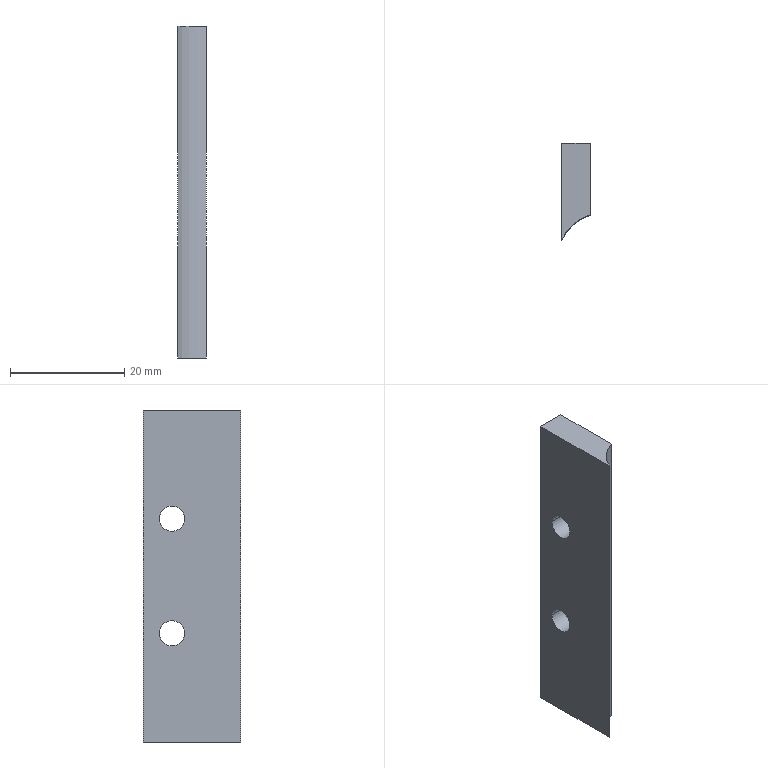Part | SolidWorks | features Extrusion 1, ICE 1 | 1 solid | 10 faces | box 5 x 17 x 58 mm | volume 3929 mm3 | cylinder 5 | plane 5 | commonest cylinder face diameters 4.4 x4 15.6 x1
STEP:
#1=CARTESIAN_POINT('',(-3.012,-2.658,19.));
#2=VERTEX_POINT('',#1);
#3=CARTESIAN_POINT('',(-3.012,1.742,19.));
#4=VERTEX_POINT('',#3);
#5=CARTESIAN_POINT('',(-3.012,-0.4585,19.));
#6=DIRECTION('',(1.,0.,0.));
#7=DIRECTION('',(0.,1.,0.));
#8=AXIS2_PLACEMENT_3D('',#5,#6,#7);
#9=CIRCLE('',#8,2.2);
#10=EDGE_CURVE('',#2,#4,#9,.T.);
#11=ORIENTED_EDGE('',*,*,#10,.F.);
#12=CARTESIAN_POINT('',(1.988,-2.658,19.));
#13=VERTEX_POINT('',#12);
#14=CARTESIAN_POINT('',(-8.012,-2.658,19.));
#15=DIRECTION('',(1.,0.,0.));
#16=VECTOR('',#15,1000.);
#17=LINE('',#14,#16);
#18=EDGE_CURVE('',#2,#13,#17,.T.);
#19=ORIENTED_EDGE('',*,*,#18,.T.);
#20=CARTESIAN_POINT('',(1.988,1.742,19.));
#21=VERTEX_POINT('',#20);
#22=CARTESIAN_POINT('',(1.988,-0.4585,19.));
#23=DIRECTION('',(1.,0.,0.));
#24=DIRECTION('',(0.,1.,0.));
#25=AXIS2_PLACEMENT_3D('',#22,#23,#24);
#26=CIRCLE('',#25,2.2);
#27=EDGE_CURVE('',#13,#21,#26,.T.);
#28=ORIENTED_EDGE('',*,*,#27,.T.);
#29=CARTESIAN_POINT('',(-8.012,1.742,19.));
#30=DIRECTION('',(1.,0.,0.));
#31=VECTOR('',#30,1000.);
#32=LINE('',#29,#31);
#33=EDGE_CURVE('',#4,#21,#32,.T.);
#34=ORIENTED_EDGE('',*,*,#33,.F.);
#35=EDGE_LOOP('',(#11,#19,#28,#34));
#36=FACE_OUTER_BOUND('',#35,.T.);
#37=CARTESIAN_POINT('',(-8.012,-0.4585,19.));
#38=DIRECTION('',(1.,0.,0.));
#39=DIRECTION('',(0.,1.,0.));
#40=AXIS2_PLACEMENT_3D('',#37,#38,#39);
#41=CYLINDRICAL_SURFACE('',#40,2.2);
#42=ADVANCED_FACE('',(#36),#41,.F.);
#43=CARTESIAN_POINT('',(-3.012,-2.658,39.));
#44=VERTEX_POINT('',#43);
#45=CARTESIAN_POINT('',(-3.012,1.742,39.));
#46=VERTEX_POINT('',#45);
#47=CARTESIAN_POINT('',(-3.012,-0.4585,39.));
#48=DIRECTION('',(1.,0.,0.));
#49=DIRECTION('',(0.,1.,0.));
#50=AXIS2_PLACEMENT_3D('',#47,#48,#49);
#51=CIRCLE('',#50,2.2);
#52=EDGE_CURVE('',#44,#46,#51,.T.);
#53=ORIENTED_EDGE('',*,*,#52,.F.);
#54=CARTESIAN_POINT('',(1.988,-2.658,39.));
#55=VERTEX_POINT('',#54);
#56=CARTESIAN_POINT('',(-8.012,-2.658,39.));
#57=DIRECTION('',(1.,0.,0.));
#58=VECTOR('',#57,1000.);
#59=LINE('',#56,#58);
#60=EDGE_CURVE('',#44,#55,#59,.T.);
#61=ORIENTED_EDGE('',*,*,#60,.T.);
#62=CARTESIAN_POINT('',(1.988,1.742,39.));
#63=VERTEX_POINT('',#62);
#64=CARTESIAN_POINT('',(1.988,-0.4585,39.));
#65=DIRECTION('',(1.,0.,0.));
#66=DIRECTION('',(0.,1.,0.));
#67=AXIS2_PLACEMENT_3D('',#64,#65,#66);
#68=CIRCLE('',#67,2.2);
#69=EDGE_CURVE('',#55,#63,#68,.T.);
#70=ORIENTED_EDGE('',*,*,#69,.T.);
#71=CARTESIAN_POINT('',(-8.012,1.742,39.));
#72=DIRECTION('',(1.,0.,0.));
#73=VECTOR('',#72,1000.);
#74=LINE('',#71,#73);
#75=EDGE_CURVE('',#46,#63,#74,.T.);
#76=ORIENTED_EDGE('',*,*,#75,.F.);
#77=EDGE_LOOP('',(#53,#61,#70,#76));
#78=FACE_OUTER_BOUND('',#77,.T.);
#79=CARTESIAN_POINT('',(-8.012,-0.4585,39.));
#80=DIRECTION('',(1.,0.,0.));
#81=DIRECTION('',(0.,1.,0.));
#82=AXIS2_PLACEMENT_3D('',#79,#80,#81);
#83=CYLINDRICAL_SURFACE('',#82,2.2);
#84=ADVANCED_FACE('',(#78),#83,.F.);
#85=CARTESIAN_POINT('',(-3.012,-0.4585,19.));
#86=DIRECTION('',(1.,0.,0.));
#87=DIRECTION('',(0.,1.,0.));
#88=AXIS2_PLACEMENT_3D('',#85,#86,#87);
#89=CIRCLE('',#88,2.2);
#90=EDGE_CURVE('',#4,#2,#89,.T.);
#91=ORIENTED_EDGE('',*,*,#90,.T.);
#92=ORIENTED_EDGE('',*,*,#10,.T.);
#93=EDGE_LOOP('',(#91,#92));
#94=FACE_BOUND('',#93,.T.);
#95=CARTESIAN_POINT('',(-3.012,-0.4585,39.));
#96=DIRECTION('',(1.,0.,0.));
#97=DIRECTION('',(0.,1.,0.));
#98=AXIS2_PLACEMENT_3D('',#95,#96,#97);
#99=CIRCLE('',#98,2.2);
#100=EDGE_CURVE('',#46,#44,#99,.T.);
#101=ORIENTED_EDGE('',*,*,#100,.T.);
#102=ORIENTED_EDGE('',*,*,#52,.T.);
#103=EDGE_LOOP('',(#101,#102));
#104=FACE_BOUND('',#103,.T.);
#105=CARTESIAN_POINT('',(-3.012,4.542,0.));
#106=VERTEX_POINT('',#105);
#107=CARTESIAN_POINT('',(-3.012,-12.458,0.));
#108=VERTEX_POINT('',#107);
#109=CARTESIAN_POINT('',(-3.012,4.542,0.));
#110=DIRECTION('',(0.,-1.,0.));
#111=VECTOR('',#110,1000.);
#112=LINE('',#109,#111);
#113=EDGE_CURVE('',#106,#108,#112,.T.);
#114=ORIENTED_EDGE('',*,*,#113,.T.);
#115=CARTESIAN_POINT('',(-3.012,-12.458,58.));
#116=VERTEX_POINT('',#115);
#117=CARTESIAN_POINT('',(-3.012,-12.458,58.));
#118=DIRECTION('',(0.,0.,-1.));
#119=VECTOR('',#118,1000.);
#120=LINE('',#117,#119);
#121=EDGE_CURVE('',#116,#108,#120,.T.);
#122=ORIENTED_EDGE('',*,*,#121,.F.);
#123=CARTESIAN_POINT('',(-3.012,4.542,58.));
#124=VERTEX_POINT('',#123);
#125=CARTESIAN_POINT('',(-3.012,4.542,58.));
#126=DIRECTION('',(0.,-1.,0.));
#127=VECTOR('',#126,1000.);
#128=LINE('',#125,#127);
#129=EDGE_CURVE('',#124,#116,#128,.T.);
#130=ORIENTED_EDGE('',*,*,#129,.F.);
#131=CARTESIAN_POINT('',(-3.012,4.542,58.));
#132=DIRECTION('',(0.,0.,-1.));
#133=VECTOR('',#132,1000.);
#134=LINE('',#131,#133);
#135=EDGE_CURVE('',#124,#106,#134,.T.);
#136=ORIENTED_EDGE('',*,*,#135,.T.);
#137=EDGE_LOOP('',(#114,#122,#130,#136));
#138=FACE_OUTER_BOUND('',#137,.T.);
#139=CARTESIAN_POINT('',(-3.012,4.542,58.));
#140=DIRECTION('',(1.,0.,0.));
#141=DIRECTION('',(0.,1.,0.));
#142=AXIS2_PLACEMENT_3D('',#139,#140,#141);
#143=PLANE('',#142);
#144=ADVANCED_FACE('',(#94,#104,#138),#143,.F.);
#145=CARTESIAN_POINT('',(1.988,-7.975,0.));
#146=VERTEX_POINT('',#145);
#147=CARTESIAN_POINT('',(4.188,-15.458,0.));
#148=DIRECTION('',(0.,0.,-1.));
#149=DIRECTION('',(1.,0.,0.));
#150=AXIS2_PLACEMENT_3D('',#147,#148,#149);
#151=CIRCLE('',#150,7.8);
#152=EDGE_CURVE('',#108,#146,#151,.T.);
#153=ORIENTED_EDGE('',*,*,#152,.T.);
#154=CARTESIAN_POINT('',(1.988,-7.975,58.));
#155=VERTEX_POINT('',#154);
#156=CARTESIAN_POINT('',(1.988,-7.975,58.));
#157=DIRECTION('',(0.,0.,-1.));
#158=VECTOR('',#157,1000.);
#159=LINE('',#156,#158);
#160=EDGE_CURVE('',#155,#146,#159,.T.);
#161=ORIENTED_EDGE('',*,*,#160,.F.);
#162=CARTESIAN_POINT('',(4.188,-15.458,58.));
#163=DIRECTION('',(0.,0.,-1.));
#164=DIRECTION('',(1.,0.,0.));
#165=AXIS2_PLACEMENT_3D('',#162,#163,#164);
#166=CIRCLE('',#165,7.8);
#167=EDGE_CURVE('',#116,#155,#166,.T.);
#168=ORIENTED_EDGE('',*,*,#167,.F.);
#169=ORIENTED_EDGE('',*,*,#121,.T.);
#170=EDGE_LOOP('',(#153,#161,#168,#169));
#171=FACE_OUTER_BOUND('',#170,.T.);
#172=CARTESIAN_POINT('',(4.188,-15.458,58.));
#173=DIRECTION('',(0.,0.,-1.));
#174=DIRECTION('',(-1.,0.,0.));
#175=AXIS2_PLACEMENT_3D('',#172,#173,#174);
#176=CYLINDRICAL_SURFACE('',#175,7.8);
#177=ADVANCED_FACE('',(#171),#176,.F.);
#178=CARTESIAN_POINT('',(1.988,-0.4585,19.));
#179=DIRECTION('',(1.,0.,0.));
#180=DIRECTION('',(0.,1.,0.));
#181=AXIS2_PLACEMENT_3D('',#178,#179,#180);
#182=CIRCLE('',#181,2.2);
#183=EDGE_CURVE('',#21,#13,#182,.T.);
#184=ORIENTED_EDGE('',*,*,#183,.F.);
#185=ORIENTED_EDGE('',*,*,#27,.F.);
#186=EDGE_LOOP('',(#184,#185));
#187=FACE_BOUND('',#186,.T.);
#188=CARTESIAN_POINT('',(1.988,-0.4585,39.));
#189=DIRECTION('',(1.,0.,0.));
#190=DIRECTION('',(0.,1.,0.));
#191=AXIS2_PLACEMENT_3D('',#188,#189,#190);
#192=CIRCLE('',#191,2.2);
#193=EDGE_CURVE('',#63,#55,#192,.T.);
#194=ORIENTED_EDGE('',*,*,#193,.F.);
#195=ORIENTED_EDGE('',*,*,#69,.F.);
#196=EDGE_LOOP('',(#194,#195));
#197=FACE_BOUND('',#196,.T.);
#198=CARTESIAN_POINT('',(1.988,4.542,0.));
#199=VERTEX_POINT('',#198);
#200=CARTESIAN_POINT('',(1.988,4.542,0.));
#201=DIRECTION('',(0.,1.,0.));
#202=VECTOR('',#201,1000.);
#203=LINE('',#200,#202);
#204=EDGE_CURVE('',#146,#199,#203,.T.);
#205=ORIENTED_EDGE('',*,*,#204,.T.);
#206=CARTESIAN_POINT('',(1.988,4.542,58.));
#207=VERTEX_POINT('',#206);
#208=CARTESIAN_POINT('',(1.988,4.542,58.));
#209=DIRECTION('',(0.,0.,-1.));
#210=VECTOR('',#209,1000.);
#211=LINE('',#208,#210);
#212=EDGE_CURVE('',#207,#199,#211,.T.);
#213=ORIENTED_EDGE('',*,*,#212,.F.);
#214=CARTESIAN_POINT('',(1.988,4.542,58.));
#215=DIRECTION('',(0.,1.,0.));
#216=VECTOR('',#215,1000.);
#217=LINE('',#214,#216);
#218=EDGE_CURVE('',#155,#207,#217,.T.);
#219=ORIENTED_EDGE('',*,*,#218,.F.);
#220=ORIENTED_EDGE('',*,*,#160,.T.);
#221=EDGE_LOOP('',(#205,#213,#219,#220));
#222=FACE_OUTER_BOUND('',#221,.T.);
#223=CARTESIAN_POINT('',(1.988,4.542,58.));
#224=DIRECTION('',(-1.,0.,0.));
#225=DIRECTION('',(0.,-1.,0.));
#226=AXIS2_PLACEMENT_3D('',#223,#224,#225);
#227=PLANE('',#226);
#228=ADVANCED_FACE('',(#187,#197,#222),#227,.F.);
#229=CARTESIAN_POINT('',(-3.012,4.542,0.));
#230=DIRECTION('',(-1.,0.,0.));
#231=VECTOR('',#230,1000.);
#232=LINE('',#229,#231);
#233=EDGE_CURVE('',#199,#106,#232,.T.);
#234=ORIENTED_EDGE('',*,*,#233,.T.);
#235=ORIENTED_EDGE('',*,*,#135,.F.);
#236=CARTESIAN_POINT('',(-3.012,4.542,58.));
#237=DIRECTION('',(-1.,0.,0.));
#238=VECTOR('',#237,1000.);
#239=LINE('',#236,#238);
#240=EDGE_CURVE('',#207,#124,#239,.T.);
#241=ORIENTED_EDGE('',*,*,#240,.F.);
#242=ORIENTED_EDGE('',*,*,#212,.T.);
#243=EDGE_LOOP('',(#234,#235,#241,#242));
#244=FACE_OUTER_BOUND('',#243,.T.);
#245=CARTESIAN_POINT('',(-3.012,4.542,58.));
#246=DIRECTION('',(0.,-1.,0.));
#247=DIRECTION('',(0.,0.,-1.));
#248=AXIS2_PLACEMENT_3D('',#245,#246,#247);
#249=PLANE('',#248);
#250=ADVANCED_FACE('',(#244),#249,.F.);
#251=ORIENTED_EDGE('',*,*,#129,.T.);
#252=ORIENTED_EDGE('',*,*,#167,.T.);
#253=ORIENTED_EDGE('',*,*,#218,.T.);
#254=ORIENTED_EDGE('',*,*,#240,.T.);
#255=EDGE_LOOP('',(#251,#252,#253,#254));
#256=FACE_OUTER_BOUND('',#255,.T.);
#257=CARTESIAN_POINT('',(4.188,-15.458,58.));
#258=DIRECTION('',(0.,0.,1.));
#259=DIRECTION('',(1.,0.,0.));
#260=AXIS2_PLACEMENT_3D('',#257,#258,#259);
#261=PLANE('',#260);
#262=ADVANCED_FACE('',(#256),#261,.T.);
#263=ORIENTED_EDGE('',*,*,#113,.F.);
#264=ORIENTED_EDGE('',*,*,#233,.F.);
#265=ORIENTED_EDGE('',*,*,#204,.F.);
#266=ORIENTED_EDGE('',*,*,#152,.F.);
#267=EDGE_LOOP('',(#263,#264,#265,#266));
#268=FACE_OUTER_BOUND('',#267,.T.);
#269=CARTESIAN_POINT('',(4.188,-15.458,0.));
#270=DIRECTION('',(0.,0.,1.));
#271=DIRECTION('',(1.,0.,0.));
#272=AXIS2_PLACEMENT_3D('',#269,#270,#271);
#273=PLANE('',#272);
#274=ADVANCED_FACE('',(#268),#273,.F.);
#275=ORIENTED_EDGE('',*,*,#60,.F.);
#276=ORIENTED_EDGE('',*,*,#100,.F.);
#277=ORIENTED_EDGE('',*,*,#75,.T.);
#278=ORIENTED_EDGE('',*,*,#193,.T.);
#279=EDGE_LOOP('',(#275,#276,#277,#278));
#280=FACE_OUTER_BOUND('',#279,.T.);
#281=CARTESIAN_POINT('',(-8.012,-0.4585,39.));
#282=DIRECTION('',(1.,0.,0.));
#283=DIRECTION('',(0.,1.,0.));
#284=AXIS2_PLACEMENT_3D('',#281,#282,#283);
#285=CYLINDRICAL_SURFACE('',#284,2.2);
#286=ADVANCED_FACE('',(#280),#285,.F.);
#287=ORIENTED_EDGE('',*,*,#18,.F.);
#288=ORIENTED_EDGE('',*,*,#90,.F.);
#289=ORIENTED_EDGE('',*,*,#33,.T.);
#290=ORIENTED_EDGE('',*,*,#183,.T.);
#291=EDGE_LOOP('',(#287,#288,#289,#290));
#292=FACE_OUTER_BOUND('',#291,.T.);
#293=CARTESIAN_POINT('',(-8.012,-0.4585,19.));
#294=DIRECTION('',(1.,0.,0.));
#295=DIRECTION('',(0.,1.,0.));
#296=AXIS2_PLACEMENT_3D('',#293,#294,#295);
#297=CYLINDRICAL_SURFACE('',#296,2.2);
#298=ADVANCED_FACE('',(#292),#297,.F.);
#299=CLOSED_SHELL('',(#42,#84,#144,#177,#228,#250,#262,#274,#286,#298));
#300=MANIFOLD_SOLID_BREP('',#299);
#301=CARTESIAN_POINT('',(0.,0.,0.));
#302=DIRECTION('',(0.,0.,1.));
#303=DIRECTION('',(1.,0.,0.));
#304=AXIS2_PLACEMENT_3D('',#301,#302,#303);
#305=(LENGTH_UNIT()NAMED_UNIT(*)SI_UNIT(.MILLI.,.METRE.));
#306=UNCERTAINTY_MEASURE_WITH_UNIT(LENGTH_MEASURE(0.00001),#305,'','');
#307=(NAMED_UNIT(*)PLANE_ANGLE_UNIT()SI_UNIT($,.RADIAN.));
#308=(NAMED_UNIT(*)SI_UNIT($,.STERADIAN.)SOLID_ANGLE_UNIT());
#309=(GEOMETRIC_REPRESENTATION_CONTEXT(3)GLOBAL_UNCERTAINTY_ASSIGNED_CONTEXT((#306))GLOBAL_UNIT_ASSIGNED_CONTEXT((#305,#307,#308))REPRESENTATION_CONTEXT('',''));
#310=ADVANCED_BREP_SHAPE_REPRESENTATION('',(#300,#304),#309);